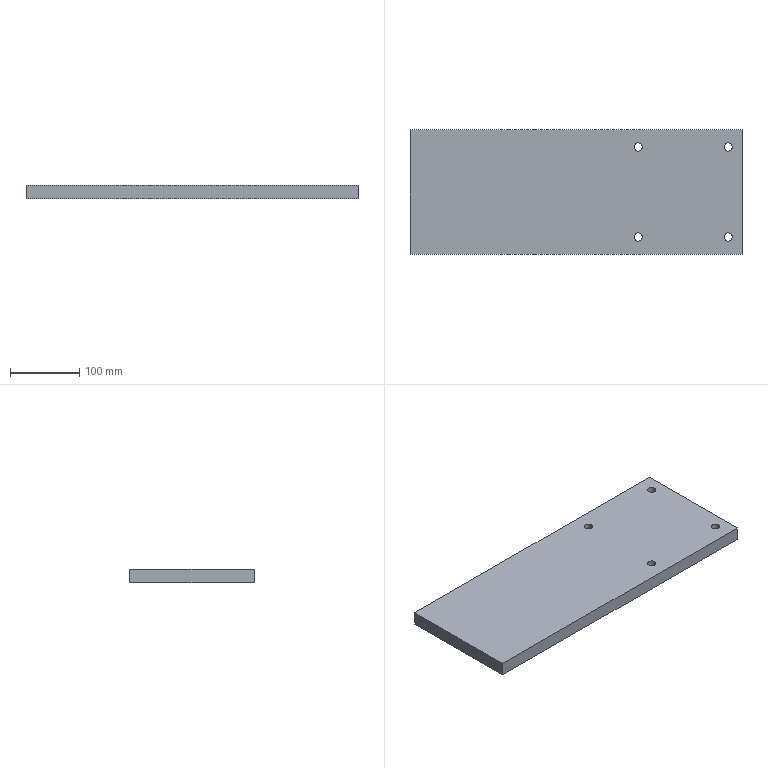Part | STEP file | Small Pad Plate 1 | 1 solid | 14 faces | box 480 x 180 x 20 mm | volume 1718952 mm3 | cylinder 8 | plane 6 | commonest cylinder face diameters 12 x8
STEP:
#1=CARTESIAN_POINT('',(0.,0.,0.));
#2=DIRECTION('',(0.,0.,1.));
#3=DIRECTION('',(1.,0.,0.));
#4=AXIS2_PLACEMENT_3D('',#1,#2,#3);
#5=CARTESIAN_POINT('',(96.,-65.,0.));
#6=VERTEX_POINT('',#5);
#7=CARTESIAN_POINT('',(96.,-65.,20.));
#8=VERTEX_POINT('',#7);
#9=CARTESIAN_POINT('',(96.,-65.,20.));
#10=DIRECTION('',(0.,0.,1.));
#11=VECTOR('',#10,1.);
#12=LINE('',#9,#11);
#13=CARTESIAN_POINT('',(90.,-65.,20.));
#14=DIRECTION('',(0.,0.,1.));
#15=DIRECTION('',(1.,0.,0.));
#16=AXIS2_PLACEMENT_3D('',#13,#14,#15);
#17=CYLINDRICAL_SURFACE('',#16,6.);
#18=CARTESIAN_POINT('',(6.283,0.));
#19=DIRECTION('',(0.,1.));
#20=VECTOR('',#19,1.);
#21=LINE('',#18,#20);
#22=(GEOMETRIC_REPRESENTATION_CONTEXT(2)PARAMETRIC_REPRESENTATION_CONTEXT()REPRESENTATION_CONTEXT('',''));
#23=DEFINITIONAL_REPRESENTATION('',(#21),#22);
#24=PCURVE('',#17,#23);
#25=CARTESIAN_POINT('',(90.,-65.,20.));
#26=DIRECTION('',(0.,0.,1.));
#27=DIRECTION('',(1.,0.,0.));
#28=AXIS2_PLACEMENT_3D('',#25,#26,#27);
#29=CYLINDRICAL_SURFACE('',#28,6.);
#30=CARTESIAN_POINT('',(0.,0.));
#31=DIRECTION('',(0.,1.));
#32=VECTOR('',#31,1.);
#33=LINE('',#30,#32);
#34=(GEOMETRIC_REPRESENTATION_CONTEXT(2)PARAMETRIC_REPRESENTATION_CONTEXT()REPRESENTATION_CONTEXT('',''));
#35=DEFINITIONAL_REPRESENTATION('',(#33),#34);
#36=PCURVE('',#29,#35);
#37=SURFACE_CURVE('',#12,(#24,#36),.PCURVE_S1.);
#38=EDGE_CURVE('',#6,#8,#37,.T.);
#39=ORIENTED_EDGE('',*,*,#38,.T.);
#40=CARTESIAN_POINT('',(84.,-65.,20.));
#41=VERTEX_POINT('',#40);
#42=CARTESIAN_POINT('',(90.,-65.,20.));
#43=DIRECTION('',(0.,0.,1.));
#44=DIRECTION('',(1.,0.,0.));
#45=AXIS2_PLACEMENT_3D('',#42,#43,#44);
#46=CIRCLE('',#45,6.);
#47=CARTESIAN_POINT('',(0.,0.));
#48=DIRECTION('',(1.,0.));
#49=VECTOR('',#48,1.);
#50=LINE('',#47,#49);
#51=(GEOMETRIC_REPRESENTATION_CONTEXT(2)PARAMETRIC_REPRESENTATION_CONTEXT()REPRESENTATION_CONTEXT('',''));
#52=DEFINITIONAL_REPRESENTATION('',(#50),#51);
#53=PCURVE('',#17,#52);
#54=CARTESIAN_POINT('',(0.,0.,20.));
#55=DIRECTION('',(0.,0.,1.));
#56=DIRECTION('',(1.,0.,0.));
#57=AXIS2_PLACEMENT_3D('',#54,#55,#56);
#58=PLANE('',#57);
#59=CARTESIAN_POINT('',(90.,-65.));
#60=DIRECTION('',(1.,0.));
#61=AXIS2_PLACEMENT_2D('',#59,#60);
#62=CIRCLE('',#61,6.);
#63=(GEOMETRIC_REPRESENTATION_CONTEXT(2)PARAMETRIC_REPRESENTATION_CONTEXT()REPRESENTATION_CONTEXT('',''));
#64=DEFINITIONAL_REPRESENTATION('',(#62),#63);
#65=PCURVE('',#58,#64);
#66=SURFACE_CURVE('',#46,(#53,#65),.PCURVE_S1.);
#67=EDGE_CURVE('',#41,#8,#66,.T.);
#68=ORIENTED_EDGE('',*,*,#67,.F.);
#69=CARTESIAN_POINT('',(84.,-65.,0.));
#70=VERTEX_POINT('',#69);
#71=CARTESIAN_POINT('',(84.,-65.,20.));
#72=DIRECTION('',(0.,0.,1.));
#73=VECTOR('',#72,1.);
#74=LINE('',#71,#73);
#75=CARTESIAN_POINT('',(3.142,0.));
#76=DIRECTION('',(0.,1.));
#77=VECTOR('',#76,1.);
#78=LINE('',#75,#77);
#79=(GEOMETRIC_REPRESENTATION_CONTEXT(2)PARAMETRIC_REPRESENTATION_CONTEXT()REPRESENTATION_CONTEXT('',''));
#80=DEFINITIONAL_REPRESENTATION('',(#78),#79);
#81=PCURVE('',#17,#80);
#82=CARTESIAN_POINT('',(3.142,0.));
#83=DIRECTION('',(0.,1.));
#84=VECTOR('',#83,1.);
#85=LINE('',#82,#84);
#86=(GEOMETRIC_REPRESENTATION_CONTEXT(2)PARAMETRIC_REPRESENTATION_CONTEXT()REPRESENTATION_CONTEXT('',''));
#87=DEFINITIONAL_REPRESENTATION('',(#85),#86);
#88=PCURVE('',#29,#87);
#89=SURFACE_CURVE('',#74,(#81,#88),.PCURVE_S1.);
#90=EDGE_CURVE('',#70,#41,#89,.T.);
#91=ORIENTED_EDGE('',*,*,#90,.F.);
#92=CARTESIAN_POINT('',(90.,-65.,0.));
#93=DIRECTION('',(0.,0.,1.));
#94=DIRECTION('',(1.,0.,0.));
#95=AXIS2_PLACEMENT_3D('',#92,#93,#94);
#96=CIRCLE('',#95,6.);
#97=CARTESIAN_POINT('',(0.,-20.));
#98=DIRECTION('',(1.,0.));
#99=VECTOR('',#98,1.);
#100=LINE('',#97,#99);
#101=(GEOMETRIC_REPRESENTATION_CONTEXT(2)PARAMETRIC_REPRESENTATION_CONTEXT()REPRESENTATION_CONTEXT('',''));
#102=DEFINITIONAL_REPRESENTATION('',(#100),#101);
#103=PCURVE('',#17,#102);
#104=CARTESIAN_POINT('',(0.,0.,0.));
#105=DIRECTION('',(0.,0.,1.));
#106=DIRECTION('',(1.,0.,0.));
#107=AXIS2_PLACEMENT_3D('',#104,#105,#106);
#108=PLANE('',#107);
#109=CARTESIAN_POINT('',(90.,-65.));
#110=DIRECTION('',(1.,0.));
#111=AXIS2_PLACEMENT_2D('',#109,#110);
#112=CIRCLE('',#111,6.);
#113=(GEOMETRIC_REPRESENTATION_CONTEXT(2)PARAMETRIC_REPRESENTATION_CONTEXT()REPRESENTATION_CONTEXT('',''));
#114=DEFINITIONAL_REPRESENTATION('',(#112),#113);
#115=PCURVE('',#108,#114);
#116=SURFACE_CURVE('',#96,(#103,#115),.PCURVE_S1.);
#117=EDGE_CURVE('',#70,#6,#116,.T.);
#118=ORIENTED_EDGE('',*,*,#117,.T.);
#119=EDGE_LOOP('',(#39,#68,#91,#118));
#120=FACE_BOUND('',#119,.F.);
#121=ADVANCED_FACE('',(#120),#17,.F.);
#122=CARTESIAN_POINT('',(96.,65.,0.));
#123=VERTEX_POINT('',#122);
#124=CARTESIAN_POINT('',(96.,65.,20.));
#125=VERTEX_POINT('',#124);
#126=CARTESIAN_POINT('',(96.,65.,20.));
#127=DIRECTION('',(0.,0.,1.));
#128=VECTOR('',#127,1.);
#129=LINE('',#126,#128);
#130=CARTESIAN_POINT('',(90.,65.,20.));
#131=DIRECTION('',(0.,0.,1.));
#132=DIRECTION('',(1.,0.,0.));
#133=AXIS2_PLACEMENT_3D('',#130,#131,#132);
#134=CYLINDRICAL_SURFACE('',#133,6.);
#135=CARTESIAN_POINT('',(6.283,0.));
#136=DIRECTION('',(0.,1.));
#137=VECTOR('',#136,1.);
#138=LINE('',#135,#137);
#139=(GEOMETRIC_REPRESENTATION_CONTEXT(2)PARAMETRIC_REPRESENTATION_CONTEXT()REPRESENTATION_CONTEXT('',''));
#140=DEFINITIONAL_REPRESENTATION('',(#138),#139);
#141=PCURVE('',#134,#140);
#142=CARTESIAN_POINT('',(90.,65.,20.));
#143=DIRECTION('',(0.,0.,1.));
#144=DIRECTION('',(1.,0.,0.));
#145=AXIS2_PLACEMENT_3D('',#142,#143,#144);
#146=CYLINDRICAL_SURFACE('',#145,6.);
#147=CARTESIAN_POINT('',(0.,0.));
#148=DIRECTION('',(0.,1.));
#149=VECTOR('',#148,1.);
#150=LINE('',#147,#149);
#151=(GEOMETRIC_REPRESENTATION_CONTEXT(2)PARAMETRIC_REPRESENTATION_CONTEXT()REPRESENTATION_CONTEXT('',''));
#152=DEFINITIONAL_REPRESENTATION('',(#150),#151);
#153=PCURVE('',#146,#152);
#154=SURFACE_CURVE('',#129,(#141,#153),.PCURVE_S1.);
#155=EDGE_CURVE('',#123,#125,#154,.T.);
#156=ORIENTED_EDGE('',*,*,#155,.T.);
#157=CARTESIAN_POINT('',(84.,65.,20.));
#158=VERTEX_POINT('',#157);
#159=CARTESIAN_POINT('',(90.,65.,20.));
#160=DIRECTION('',(0.,0.,1.));
#161=DIRECTION('',(1.,0.,0.));
#162=AXIS2_PLACEMENT_3D('',#159,#160,#161);
#163=CIRCLE('',#162,6.);
#164=CARTESIAN_POINT('',(0.,0.));
#165=DIRECTION('',(1.,0.));
#166=VECTOR('',#165,1.);
#167=LINE('',#164,#166);
#168=(GEOMETRIC_REPRESENTATION_CONTEXT(2)PARAMETRIC_REPRESENTATION_CONTEXT()REPRESENTATION_CONTEXT('',''));
#169=DEFINITIONAL_REPRESENTATION('',(#167),#168);
#170=PCURVE('',#134,#169);
#171=CARTESIAN_POINT('',(90.,65.));
#172=DIRECTION('',(1.,0.));
#173=AXIS2_PLACEMENT_2D('',#171,#172);
#174=CIRCLE('',#173,6.);
#175=(GEOMETRIC_REPRESENTATION_CONTEXT(2)PARAMETRIC_REPRESENTATION_CONTEXT()REPRESENTATION_CONTEXT('',''));
#176=DEFINITIONAL_REPRESENTATION('',(#174),#175);
#177=PCURVE('',#58,#176);
#178=SURFACE_CURVE('',#163,(#170,#177),.PCURVE_S1.);
#179=EDGE_CURVE('',#158,#125,#178,.T.);
#180=ORIENTED_EDGE('',*,*,#179,.F.);
#181=CARTESIAN_POINT('',(84.,65.,0.));
#182=VERTEX_POINT('',#181);
#183=CARTESIAN_POINT('',(84.,65.,20.));
#184=DIRECTION('',(0.,0.,1.));
#185=VECTOR('',#184,1.);
#186=LINE('',#183,#185);
#187=CARTESIAN_POINT('',(3.142,0.));
#188=DIRECTION('',(0.,1.));
#189=VECTOR('',#188,1.);
#190=LINE('',#187,#189);
#191=(GEOMETRIC_REPRESENTATION_CONTEXT(2)PARAMETRIC_REPRESENTATION_CONTEXT()REPRESENTATION_CONTEXT('',''));
#192=DEFINITIONAL_REPRESENTATION('',(#190),#191);
#193=PCURVE('',#134,#192);
#194=CARTESIAN_POINT('',(3.142,0.));
#195=DIRECTION('',(0.,1.));
#196=VECTOR('',#195,1.);
#197=LINE('',#194,#196);
#198=(GEOMETRIC_REPRESENTATION_CONTEXT(2)PARAMETRIC_REPRESENTATION_CONTEXT()REPRESENTATION_CONTEXT('',''));
#199=DEFINITIONAL_REPRESENTATION('',(#197),#198);
#200=PCURVE('',#146,#199);
#201=SURFACE_CURVE('',#186,(#193,#200),.PCURVE_S1.);
#202=EDGE_CURVE('',#182,#158,#201,.T.);
#203=ORIENTED_EDGE('',*,*,#202,.F.);
#204=CARTESIAN_POINT('',(90.,65.,0.));
#205=DIRECTION('',(0.,0.,1.));
#206=DIRECTION('',(1.,0.,0.));
#207=AXIS2_PLACEMENT_3D('',#204,#205,#206);
#208=CIRCLE('',#207,6.);
#209=CARTESIAN_POINT('',(0.,-20.));
#210=DIRECTION('',(1.,0.));
#211=VECTOR('',#210,1.);
#212=LINE('',#209,#211);
#213=(GEOMETRIC_REPRESENTATION_CONTEXT(2)PARAMETRIC_REPRESENTATION_CONTEXT()REPRESENTATION_CONTEXT('',''));
#214=DEFINITIONAL_REPRESENTATION('',(#212),#213);
#215=PCURVE('',#134,#214);
#216=CARTESIAN_POINT('',(90.,65.));
#217=DIRECTION('',(1.,0.));
#218=AXIS2_PLACEMENT_2D('',#216,#217);
#219=CIRCLE('',#218,6.);
#220=(GEOMETRIC_REPRESENTATION_CONTEXT(2)PARAMETRIC_REPRESENTATION_CONTEXT()REPRESENTATION_CONTEXT('',''));
#221=DEFINITIONAL_REPRESENTATION('',(#219),#220);
#222=PCURVE('',#108,#221);
#223=SURFACE_CURVE('',#208,(#215,#222),.PCURVE_S1.);
#224=EDGE_CURVE('',#182,#123,#223,.T.);
#225=ORIENTED_EDGE('',*,*,#224,.T.);
#226=EDGE_LOOP('',(#156,#180,#203,#225));
#227=FACE_BOUND('',#226,.F.);
#228=ADVANCED_FACE('',(#227),#134,.F.);
#229=CARTESIAN_POINT('',(226.,-65.,0.));
#230=VERTEX_POINT('',#229);
#231=CARTESIAN_POINT('',(226.,-65.,20.));
#232=VERTEX_POINT('',#231);
#233=CARTESIAN_POINT('',(226.,-65.,20.));
#234=DIRECTION('',(0.,0.,1.));
#235=VECTOR('',#234,1.);
#236=LINE('',#233,#235);
#237=CARTESIAN_POINT('',(220.,-65.,20.));
#238=DIRECTION('',(0.,0.,1.));
#239=DIRECTION('',(1.,0.,0.));
#240=AXIS2_PLACEMENT_3D('',#237,#238,#239);
#241=CYLINDRICAL_SURFACE('',#240,6.);
#242=CARTESIAN_POINT('',(6.283,0.));
#243=DIRECTION('',(0.,1.));
#244=VECTOR('',#243,1.);
#245=LINE('',#242,#244);
#246=(GEOMETRIC_REPRESENTATION_CONTEXT(2)PARAMETRIC_REPRESENTATION_CONTEXT()REPRESENTATION_CONTEXT('',''));
#247=DEFINITIONAL_REPRESENTATION('',(#245),#246);
#248=PCURVE('',#241,#247);
#249=CARTESIAN_POINT('',(220.,-65.,20.));
#250=DIRECTION('',(0.,0.,1.));
#251=DIRECTION('',(1.,0.,0.));
#252=AXIS2_PLACEMENT_3D('',#249,#250,#251);
#253=CYLINDRICAL_SURFACE('',#252,6.);
#254=CARTESIAN_POINT('',(0.,0.));
#255=DIRECTION('',(0.,1.));
#256=VECTOR('',#255,1.);
#257=LINE('',#254,#256);
#258=(GEOMETRIC_REPRESENTATION_CONTEXT(2)PARAMETRIC_REPRESENTATION_CONTEXT()REPRESENTATION_CONTEXT('',''));
#259=DEFINITIONAL_REPRESENTATION('',(#257),#258);
#260=PCURVE('',#253,#259);
#261=SURFACE_CURVE('',#236,(#248,#260),.PCURVE_S1.);
#262=EDGE_CURVE('',#230,#232,#261,.T.);
#263=ORIENTED_EDGE('',*,*,#262,.T.);
#264=CARTESIAN_POINT('',(214.,-65.,20.));
#265=VERTEX_POINT('',#264);
#266=CARTESIAN_POINT('',(220.,-65.,20.));
#267=DIRECTION('',(0.,0.,1.));
#268=DIRECTION('',(1.,0.,0.));
#269=AXIS2_PLACEMENT_3D('',#266,#267,#268);
#270=CIRCLE('',#269,6.);
#271=CARTESIAN_POINT('',(0.,0.));
#272=DIRECTION('',(1.,0.));
#273=VECTOR('',#272,1.);
#274=LINE('',#271,#273);
#275=(GEOMETRIC_REPRESENTATION_CONTEXT(2)PARAMETRIC_REPRESENTATION_CONTEXT()REPRESENTATION_CONTEXT('',''));
#276=DEFINITIONAL_REPRESENTATION('',(#274),#275);
#277=PCURVE('',#241,#276);
#278=CARTESIAN_POINT('',(220.,-65.));
#279=DIRECTION('',(1.,0.));
#280=AXIS2_PLACEMENT_2D('',#278,#279);
#281=CIRCLE('',#280,6.);
#282=(GEOMETRIC_REPRESENTATION_CONTEXT(2)PARAMETRIC_REPRESENTATION_CONTEXT()REPRESENTATION_CONTEXT('',''));
#283=DEFINITIONAL_REPRESENTATION('',(#281),#282);
#284=PCURVE('',#58,#283);
#285=SURFACE_CURVE('',#270,(#277,#284),.PCURVE_S1.);
#286=EDGE_CURVE('',#265,#232,#285,.T.);
#287=ORIENTED_EDGE('',*,*,#286,.F.);
#288=CARTESIAN_POINT('',(214.,-65.,0.));
#289=VERTEX_POINT('',#288);
#290=CARTESIAN_POINT('',(214.,-65.,20.));
#291=DIRECTION('',(0.,0.,1.));
#292=VECTOR('',#291,1.);
#293=LINE('',#290,#292);
#294=CARTESIAN_POINT('',(3.142,0.));
#295=DIRECTION('',(0.,1.));
#296=VECTOR('',#295,1.);
#297=LINE('',#294,#296);
#298=(GEOMETRIC_REPRESENTATION_CONTEXT(2)PARAMETRIC_REPRESENTATION_CONTEXT()REPRESENTATION_CONTEXT('',''));
#299=DEFINITIONAL_REPRESENTATION('',(#297),#298);
#300=PCURVE('',#241,#299);
#301=CARTESIAN_POINT('',(3.142,0.));
#302=DIRECTION('',(0.,1.));
#303=VECTOR('',#302,1.);
#304=LINE('',#301,#303);
#305=(GEOMETRIC_REPRESENTATION_CONTEXT(2)PARAMETRIC_REPRESENTATION_CONTEXT()REPRESENTATION_CONTEXT('',''));
#306=DEFINITIONAL_REPRESENTATION('',(#304),#305);
#307=PCURVE('',#253,#306);
#308=SURFACE_CURVE('',#293,(#300,#307),.PCURVE_S1.);
#309=EDGE_CURVE('',#289,#265,#308,.T.);
#310=ORIENTED_EDGE('',*,*,#309,.F.);
#311=CARTESIAN_POINT('',(220.,-65.,0.));
#312=DIRECTION('',(0.,0.,1.));
#313=DIRECTION('',(1.,0.,0.));
#314=AXIS2_PLACEMENT_3D('',#311,#312,#313);
#315=CIRCLE('',#314,6.);
#316=CARTESIAN_POINT('',(0.,-20.));
#317=DIRECTION('',(1.,0.));
#318=VECTOR('',#317,1.);
#319=LINE('',#316,#318);
#320=(GEOMETRIC_REPRESENTATION_CONTEXT(2)PARAMETRIC_REPRESENTATION_CONTEXT()REPRESENTATION_CONTEXT('',''));
#321=DEFINITIONAL_REPRESENTATION('',(#319),#320);
#322=PCURVE('',#241,#321);
#323=CARTESIAN_POINT('',(220.,-65.));
#324=DIRECTION('',(1.,0.));
#325=AXIS2_PLACEMENT_2D('',#323,#324);
#326=CIRCLE('',#325,6.);
#327=(GEOMETRIC_REPRESENTATION_CONTEXT(2)PARAMETRIC_REPRESENTATION_CONTEXT()REPRESENTATION_CONTEXT('',''));
#328=DEFINITIONAL_REPRESENTATION('',(#326),#327);
#329=PCURVE('',#108,#328);
#330=SURFACE_CURVE('',#315,(#322,#329),.PCURVE_S1.);
#331=EDGE_CURVE('',#289,#230,#330,.T.);
#332=ORIENTED_EDGE('',*,*,#331,.T.);
#333=EDGE_LOOP('',(#263,#287,#310,#332));
#334=FACE_BOUND('',#333,.F.);
#335=ADVANCED_FACE('',(#334),#241,.F.);
#336=CARTESIAN_POINT('',(226.,65.,0.));
#337=VERTEX_POINT('',#336);
#338=CARTESIAN_POINT('',(226.,65.,20.));
#339=VERTEX_POINT('',#338);
#340=CARTESIAN_POINT('',(226.,65.,20.));
#341=DIRECTION('',(0.,0.,1.));
#342=VECTOR('',#341,1.);
#343=LINE('',#340,#342);
#344=CARTESIAN_POINT('',(220.,65.,20.));
#345=DIRECTION('',(0.,0.,1.));
#346=DIRECTION('',(1.,0.,0.));
#347=AXIS2_PLACEMENT_3D('',#344,#345,#346);
#348=CYLINDRICAL_SURFACE('',#347,6.);
#349=CARTESIAN_POINT('',(6.283,0.));
#350=DIRECTION('',(0.,1.));
#351=VECTOR('',#350,1.);
#352=LINE('',#349,#351);
#353=(GEOMETRIC_REPRESENTATION_CONTEXT(2)PARAMETRIC_REPRESENTATION_CONTEXT()REPRESENTATION_CONTEXT('',''));
#354=DEFINITIONAL_REPRESENTATION('',(#352),#353);
#355=PCURVE('',#348,#354);
#356=CARTESIAN_POINT('',(220.,65.,20.));
#357=DIRECTION('',(0.,0.,1.));
#358=DIRECTION('',(1.,0.,0.));
#359=AXIS2_PLACEMENT_3D('',#356,#357,#358);
#360=CYLINDRICAL_SURFACE('',#359,6.);
#361=CARTESIAN_POINT('',(0.,0.));
#362=DIRECTION('',(0.,1.));
#363=VECTOR('',#362,1.);
#364=LINE('',#361,#363);
#365=(GEOMETRIC_REPRESENTATION_CONTEXT(2)PARAMETRIC_REPRESENTATION_CONTEXT()REPRESENTATION_CONTEXT('',''));
#366=DEFINITIONAL_REPRESENTATION('',(#364),#365);
#367=PCURVE('',#360,#366);
#368=SURFACE_CURVE('',#343,(#355,#367),.PCURVE_S1.);
#369=EDGE_CURVE('',#337,#339,#368,.T.);
#370=ORIENTED_EDGE('',*,*,#369,.T.);
#371=CARTESIAN_POINT('',(214.,65.,20.));
#372=VERTEX_POINT('',#371);
#373=CARTESIAN_POINT('',(220.,65.,20.));
#374=DIRECTION('',(0.,0.,1.));
#375=DIRECTION('',(1.,0.,0.));
#376=AXIS2_PLACEMENT_3D('',#373,#374,#375);
#377=CIRCLE('',#376,6.);
#378=CARTESIAN_POINT('',(0.,0.));
#379=DIRECTION('',(1.,0.));
#380=VECTOR('',#379,1.);
#381=LINE('',#378,#380);
#382=(GEOMETRIC_REPRESENTATION_CONTEXT(2)PARAMETRIC_REPRESENTATION_CONTEXT()REPRESENTATION_CONTEXT('',''));
#383=DEFINITIONAL_REPRESENTATION('',(#381),#382);
#384=PCURVE('',#348,#383);
#385=CARTESIAN_POINT('',(220.,65.));
#386=DIRECTION('',(1.,0.));
#387=AXIS2_PLACEMENT_2D('',#385,#386);
#388=CIRCLE('',#387,6.);
#389=(GEOMETRIC_REPRESENTATION_CONTEXT(2)PARAMETRIC_REPRESENTATION_CONTEXT()REPRESENTATION_CONTEXT('',''));
#390=DEFINITIONAL_REPRESENTATION('',(#388),#389);
#391=PCURVE('',#58,#390);
#392=SURFACE_CURVE('',#377,(#384,#391),.PCURVE_S1.);
#393=EDGE_CURVE('',#372,#339,#392,.T.);
#394=ORIENTED_EDGE('',*,*,#393,.F.);
#395=CARTESIAN_POINT('',(214.,65.,0.));
#396=VERTEX_POINT('',#395);
#397=CARTESIAN_POINT('',(214.,65.,20.));
#398=DIRECTION('',(0.,0.,1.));
#399=VECTOR('',#398,1.);
#400=LINE('',#397,#399);
#401=CARTESIAN_POINT('',(3.142,0.));
#402=DIRECTION('',(0.,1.));
#403=VECTOR('',#402,1.);
#404=LINE('',#401,#403);
#405=(GEOMETRIC_REPRESENTATION_CONTEXT(2)PARAMETRIC_REPRESENTATION_CONTEXT()REPRESENTATION_CONTEXT('',''));
#406=DEFINITIONAL_REPRESENTATION('',(#404),#405);
#407=PCURVE('',#348,#406);
#408=CARTESIAN_POINT('',(3.142,0.));
#409=DIRECTION('',(0.,1.));
#410=VECTOR('',#409,1.);
#411=LINE('',#408,#410);
#412=(GEOMETRIC_REPRESENTATION_CONTEXT(2)PARAMETRIC_REPRESENTATION_CONTEXT()REPRESENTATION_CONTEXT('',''));
#413=DEFINITIONAL_REPRESENTATION('',(#411),#412);
#414=PCURVE('',#360,#413);
#415=SURFACE_CURVE('',#400,(#407,#414),.PCURVE_S1.);
#416=EDGE_CURVE('',#396,#372,#415,.T.);
#417=ORIENTED_EDGE('',*,*,#416,.F.);
#418=CARTESIAN_POINT('',(220.,65.,0.));
#419=DIRECTION('',(0.,0.,1.));
#420=DIRECTION('',(1.,0.,0.));
#421=AXIS2_PLACEMENT_3D('',#418,#419,#420);
#422=CIRCLE('',#421,6.);
#423=CARTESIAN_POINT('',(0.,-20.));
#424=DIRECTION('',(1.,0.));
#425=VECTOR('',#424,1.);
#426=LINE('',#423,#425);
#427=(GEOMETRIC_REPRESENTATION_CONTEXT(2)PARAMETRIC_REPRESENTATION_CONTEXT()REPRESENTATION_CONTEXT('',''));
#428=DEFINITIONAL_REPRESENTATION('',(#426),#427);
#429=PCURVE('',#348,#428);
#430=CARTESIAN_POINT('',(220.,65.));
#431=DIRECTION('',(1.,0.));
#432=AXIS2_PLACEMENT_2D('',#430,#431);
#433=CIRCLE('',#432,6.);
#434=(GEOMETRIC_REPRESENTATION_CONTEXT(2)PARAMETRIC_REPRESENTATION_CONTEXT()REPRESENTATION_CONTEXT('',''));
#435=DEFINITIONAL_REPRESENTATION('',(#433),#434);
#436=PCURVE('',#108,#435);
#437=SURFACE_CURVE('',#422,(#429,#436),.PCURVE_S1.);
#438=EDGE_CURVE('',#396,#337,#437,.T.);
#439=ORIENTED_EDGE('',*,*,#438,.T.);
#440=EDGE_LOOP('',(#370,#394,#417,#439));
#441=FACE_BOUND('',#440,.F.);
#442=ADVANCED_FACE('',(#441),#348,.F.);
#443=CARTESIAN_POINT('',(240.,-90.,0.));
#444=VERTEX_POINT('',#443);
#445=CARTESIAN_POINT('',(240.,90.,0.));
#446=VERTEX_POINT('',#445);
#447=CARTESIAN_POINT('',(240.,90.,0.));
#448=DIRECTION('',(0.,1.,0.));
#449=VECTOR('',#448,1.);
#450=LINE('',#447,#449);
#451=CARTESIAN_POINT('',(240.,90.,20.));
#452=DIRECTION('',(-1.,0.,0.));
#453=DIRECTION('',(0.,-1.,0.));
#454=AXIS2_PLACEMENT_3D('',#451,#452,#453);
#455=PLANE('',#454);
#456=CARTESIAN_POINT('',(0.,-20.));
#457=DIRECTION('',(-1.,0.));
#458=VECTOR('',#457,1.);
#459=LINE('',#456,#458);
#460=(GEOMETRIC_REPRESENTATION_CONTEXT(2)PARAMETRIC_REPRESENTATION_CONTEXT()REPRESENTATION_CONTEXT('',''));
#461=DEFINITIONAL_REPRESENTATION('',(#459),#460);
#462=PCURVE('',#455,#461);
#463=CARTESIAN_POINT('',(240.,90.));
#464=DIRECTION('',(0.,1.));
#465=VECTOR('',#464,1.);
#466=LINE('',#463,#465);
#467=(GEOMETRIC_REPRESENTATION_CONTEXT(2)PARAMETRIC_REPRESENTATION_CONTEXT()REPRESENTATION_CONTEXT('',''));
#468=DEFINITIONAL_REPRESENTATION('',(#466),#467);
#469=PCURVE('',#108,#468);
#470=SURFACE_CURVE('',#450,(#462,#469),.PCURVE_S1.);
#471=EDGE_CURVE('',#444,#446,#470,.T.);
#472=ORIENTED_EDGE('',*,*,#471,.T.);
#473=CARTESIAN_POINT('',(240.,90.,20.));
#474=VERTEX_POINT('',#473);
#475=CARTESIAN_POINT('',(240.,90.,20.));
#476=DIRECTION('',(0.,0.,-1.));
#477=VECTOR('',#476,1.);
#478=LINE('',#475,#477);
#479=CARTESIAN_POINT('',(0.,0.));
#480=DIRECTION('',(0.,-1.));
#481=VECTOR('',#480,1.);
#482=LINE('',#479,#481);
#483=(GEOMETRIC_REPRESENTATION_CONTEXT(2)PARAMETRIC_REPRESENTATION_CONTEXT()REPRESENTATION_CONTEXT('',''));
#484=DEFINITIONAL_REPRESENTATION('',(#482),#483);
#485=PCURVE('',#455,#484);
#486=CARTESIAN_POINT('',(-240.,90.,20.));
#487=DIRECTION('',(0.,-1.,0.));
#488=DIRECTION('',(0.,0.,-1.));
#489=AXIS2_PLACEMENT_3D('',#486,#487,#488);
#490=PLANE('',#489);
#491=CARTESIAN_POINT('',(0.,480.));
#492=DIRECTION('',(1.,0.));
#493=VECTOR('',#492,1.);
#494=LINE('',#491,#493);
#495=(GEOMETRIC_REPRESENTATION_CONTEXT(2)PARAMETRIC_REPRESENTATION_CONTEXT()REPRESENTATION_CONTEXT('',''));
#496=DEFINITIONAL_REPRESENTATION('',(#494),#495);
#497=PCURVE('',#490,#496);
#498=SURFACE_CURVE('',#478,(#485,#497),.PCURVE_S1.);
#499=EDGE_CURVE('',#474,#446,#498,.T.);
#500=ORIENTED_EDGE('',*,*,#499,.F.);
#501=CARTESIAN_POINT('',(240.,-90.,20.));
#502=VERTEX_POINT('',#501);
#503=CARTESIAN_POINT('',(240.,90.,20.));
#504=DIRECTION('',(0.,1.,0.));
#505=VECTOR('',#504,1.);
#506=LINE('',#503,#505);
#507=CARTESIAN_POINT('',(0.,0.));
#508=DIRECTION('',(-1.,0.));
#509=VECTOR('',#508,1.);
#510=LINE('',#507,#509);
#511=(GEOMETRIC_REPRESENTATION_CONTEXT(2)PARAMETRIC_REPRESENTATION_CONTEXT()REPRESENTATION_CONTEXT('',''));
#512=DEFINITIONAL_REPRESENTATION('',(#510),#511);
#513=PCURVE('',#455,#512);
#514=CARTESIAN_POINT('',(240.,90.));
#515=DIRECTION('',(0.,1.));
#516=VECTOR('',#515,1.);
#517=LINE('',#514,#516);
#518=(GEOMETRIC_REPRESENTATION_CONTEXT(2)PARAMETRIC_REPRESENTATION_CONTEXT()REPRESENTATION_CONTEXT('',''));
#519=DEFINITIONAL_REPRESENTATION('',(#517),#518);
#520=PCURVE('',#58,#519);
#521=SURFACE_CURVE('',#506,(#513,#520),.PCURVE_S1.);
#522=EDGE_CURVE('',#502,#474,#521,.T.);
#523=ORIENTED_EDGE('',*,*,#522,.F.);
#524=CARTESIAN_POINT('',(240.,-90.,20.));
#525=DIRECTION('',(0.,0.,-1.));
#526=VECTOR('',#525,1.);
#527=LINE('',#524,#526);
#528=CARTESIAN_POINT('',(180.,0.));
#529=DIRECTION('',(0.,-1.));
#530=VECTOR('',#529,1.);
#531=LINE('',#528,#530);
#532=(GEOMETRIC_REPRESENTATION_CONTEXT(2)PARAMETRIC_REPRESENTATION_CONTEXT()REPRESENTATION_CONTEXT('',''));
#533=DEFINITIONAL_REPRESENTATION('',(#531),#532);
#534=PCURVE('',#455,#533);
#535=CARTESIAN_POINT('',(-240.,-90.,20.));
#536=DIRECTION('',(0.,1.,0.));
#537=DIRECTION('',(0.,0.,1.));
#538=AXIS2_PLACEMENT_3D('',#535,#536,#537);
#539=PLANE('',#538);
#540=CARTESIAN_POINT('',(0.,480.));
#541=DIRECTION('',(-1.,0.));
#542=VECTOR('',#541,1.);
#543=LINE('',#540,#542);
#544=(GEOMETRIC_REPRESENTATION_CONTEXT(2)PARAMETRIC_REPRESENTATION_CONTEXT()REPRESENTATION_CONTEXT('',''));
#545=DEFINITIONAL_REPRESENTATION('',(#543),#544);
#546=PCURVE('',#539,#545);
#547=SURFACE_CURVE('',#527,(#534,#546),.PCURVE_S1.);
#548=EDGE_CURVE('',#502,#444,#547,.T.);
#549=ORIENTED_EDGE('',*,*,#548,.T.);
#550=EDGE_LOOP('',(#472,#500,#523,#549));
#551=FACE_BOUND('',#550,.T.);
#552=ADVANCED_FACE('',(#551),#455,.F.);
#553=CARTESIAN_POINT('',(-240.,90.,0.));
#554=VERTEX_POINT('',#553);
#555=CARTESIAN_POINT('',(-240.,90.,0.));
#556=DIRECTION('',(-1.,0.,0.));
#557=VECTOR('',#556,1.);
#558=LINE('',#555,#557);
#559=CARTESIAN_POINT('',(20.,0.));
#560=DIRECTION('',(0.,-1.));
#561=VECTOR('',#560,1.);
#562=LINE('',#559,#561);
#563=(GEOMETRIC_REPRESENTATION_CONTEXT(2)PARAMETRIC_REPRESENTATION_CONTEXT()REPRESENTATION_CONTEXT('',''));
#564=DEFINITIONAL_REPRESENTATION('',(#562),#563);
#565=PCURVE('',#490,#564);
#566=CARTESIAN_POINT('',(-240.,90.));
#567=DIRECTION('',(-1.,0.));
#568=VECTOR('',#567,1.);
#569=LINE('',#566,#568);
#570=(GEOMETRIC_REPRESENTATION_CONTEXT(2)PARAMETRIC_REPRESENTATION_CONTEXT()REPRESENTATION_CONTEXT('',''));
#571=DEFINITIONAL_REPRESENTATION('',(#569),#570);
#572=PCURVE('',#108,#571);
#573=SURFACE_CURVE('',#558,(#565,#572),.PCURVE_S1.);
#574=EDGE_CURVE('',#446,#554,#573,.T.);
#575=ORIENTED_EDGE('',*,*,#574,.T.);
#576=CARTESIAN_POINT('',(-240.,90.,20.));
#577=VERTEX_POINT('',#576);
#578=CARTESIAN_POINT('',(-240.,90.,20.));
#579=DIRECTION('',(0.,0.,-1.));
#580=VECTOR('',#579,1.);
#581=LINE('',#578,#580);
#582=CARTESIAN_POINT('',(0.,0.));
#583=DIRECTION('',(1.,0.));
#584=VECTOR('',#583,1.);
#585=LINE('',#582,#584);
#586=(GEOMETRIC_REPRESENTATION_CONTEXT(2)PARAMETRIC_REPRESENTATION_CONTEXT()REPRESENTATION_CONTEXT('',''));
#587=DEFINITIONAL_REPRESENTATION('',(#585),#586);
#588=PCURVE('',#490,#587);
#589=CARTESIAN_POINT('',(-240.,90.,20.));
#590=DIRECTION('',(1.,0.,0.));
#591=DIRECTION('',(0.,1.,0.));
#592=AXIS2_PLACEMENT_3D('',#589,#590,#591);
#593=PLANE('',#592);
#594=CARTESIAN_POINT('',(0.,0.));
#595=DIRECTION('',(0.,-1.));
#596=VECTOR('',#595,1.);
#597=LINE('',#594,#596);
#598=(GEOMETRIC_REPRESENTATION_CONTEXT(2)PARAMETRIC_REPRESENTATION_CONTEXT()REPRESENTATION_CONTEXT('',''));
#599=DEFINITIONAL_REPRESENTATION('',(#597),#598);
#600=PCURVE('',#593,#599);
#601=SURFACE_CURVE('',#581,(#588,#600),.PCURVE_S1.);
#602=EDGE_CURVE('',#577,#554,#601,.T.);
#603=ORIENTED_EDGE('',*,*,#602,.F.);
#604=CARTESIAN_POINT('',(-240.,90.,20.));
#605=DIRECTION('',(-1.,0.,0.));
#606=VECTOR('',#605,1.);
#607=LINE('',#604,#606);
#608=CARTESIAN_POINT('',(0.,0.));
#609=DIRECTION('',(0.,-1.));
#610=VECTOR('',#609,1.);
#611=LINE('',#608,#610);
#612=(GEOMETRIC_REPRESENTATION_CONTEXT(2)PARAMETRIC_REPRESENTATION_CONTEXT()REPRESENTATION_CONTEXT('',''));
#613=DEFINITIONAL_REPRESENTATION('',(#611),#612);
#614=PCURVE('',#490,#613);
#615=CARTESIAN_POINT('',(-240.,90.));
#616=DIRECTION('',(-1.,0.));
#617=VECTOR('',#616,1.);
#618=LINE('',#615,#617);
#619=(GEOMETRIC_REPRESENTATION_CONTEXT(2)PARAMETRIC_REPRESENTATION_CONTEXT()REPRESENTATION_CONTEXT('',''));
#620=DEFINITIONAL_REPRESENTATION('',(#618),#619);
#621=PCURVE('',#58,#620);
#622=SURFACE_CURVE('',#607,(#614,#621),.PCURVE_S1.);
#623=EDGE_CURVE('',#474,#577,#622,.T.);
#624=ORIENTED_EDGE('',*,*,#623,.F.);
#625=ORIENTED_EDGE('',*,*,#499,.T.);
#626=EDGE_LOOP('',(#575,#603,#624,#625));
#627=FACE_BOUND('',#626,.T.);
#628=ADVANCED_FACE('',(#627),#490,.F.);
#629=CARTESIAN_POINT('',(-240.,-90.,0.));
#630=VERTEX_POINT('',#629);
#631=CARTESIAN_POINT('',(-240.,90.,0.));
#632=DIRECTION('',(0.,-1.,0.));
#633=VECTOR('',#632,1.);
#634=LINE('',#631,#633);
#635=CARTESIAN_POINT('',(0.,-20.));
#636=DIRECTION('',(-1.,0.));
#637=VECTOR('',#636,1.);
#638=LINE('',#635,#637);
#639=(GEOMETRIC_REPRESENTATION_CONTEXT(2)PARAMETRIC_REPRESENTATION_CONTEXT()REPRESENTATION_CONTEXT('',''));
#640=DEFINITIONAL_REPRESENTATION('',(#638),#639);
#641=PCURVE('',#593,#640);
#642=CARTESIAN_POINT('',(-240.,90.));
#643=DIRECTION('',(0.,-1.));
#644=VECTOR('',#643,1.);
#645=LINE('',#642,#644);
#646=(GEOMETRIC_REPRESENTATION_CONTEXT(2)PARAMETRIC_REPRESENTATION_CONTEXT()REPRESENTATION_CONTEXT('',''));
#647=DEFINITIONAL_REPRESENTATION('',(#645),#646);
#648=PCURVE('',#108,#647);
#649=SURFACE_CURVE('',#634,(#641,#648),.PCURVE_S1.);
#650=EDGE_CURVE('',#554,#630,#649,.T.);
#651=ORIENTED_EDGE('',*,*,#650,.T.);
#652=CARTESIAN_POINT('',(-240.,-90.,20.));
#653=VERTEX_POINT('',#652);
#654=CARTESIAN_POINT('',(-240.,-90.,20.));
#655=DIRECTION('',(0.,0.,-1.));
#656=VECTOR('',#655,1.);
#657=LINE('',#654,#656);
#658=CARTESIAN_POINT('',(-180.,0.));
#659=DIRECTION('',(0.,-1.));
#660=VECTOR('',#659,1.);
#661=LINE('',#658,#660);
#662=(GEOMETRIC_REPRESENTATION_CONTEXT(2)PARAMETRIC_REPRESENTATION_CONTEXT()REPRESENTATION_CONTEXT('',''));
#663=DEFINITIONAL_REPRESENTATION('',(#661),#662);
#664=PCURVE('',#593,#663);
#665=CARTESIAN_POINT('',(0.,0.));
#666=DIRECTION('',(-1.,0.));
#667=VECTOR('',#666,1.);
#668=LINE('',#665,#667);
#669=(GEOMETRIC_REPRESENTATION_CONTEXT(2)PARAMETRIC_REPRESENTATION_CONTEXT()REPRESENTATION_CONTEXT('',''));
#670=DEFINITIONAL_REPRESENTATION('',(#668),#669);
#671=PCURVE('',#539,#670);
#672=SURFACE_CURVE('',#657,(#664,#671),.PCURVE_S1.);
#673=EDGE_CURVE('',#653,#630,#672,.T.);
#674=ORIENTED_EDGE('',*,*,#673,.F.);
#675=CARTESIAN_POINT('',(-240.,90.,20.));
#676=DIRECTION('',(0.,-1.,0.));
#677=VECTOR('',#676,1.);
#678=LINE('',#675,#677);
#679=CARTESIAN_POINT('',(0.,0.));
#680=DIRECTION('',(-1.,0.));
#681=VECTOR('',#680,1.);
#682=LINE('',#679,#681);
#683=(GEOMETRIC_REPRESENTATION_CONTEXT(2)PARAMETRIC_REPRESENTATION_CONTEXT()REPRESENTATION_CONTEXT('',''));
#684=DEFINITIONAL_REPRESENTATION('',(#682),#683);
#685=PCURVE('',#593,#684);
#686=CARTESIAN_POINT('',(-240.,90.));
#687=DIRECTION('',(0.,-1.));
#688=VECTOR('',#687,1.);
#689=LINE('',#686,#688);
#690=(GEOMETRIC_REPRESENTATION_CONTEXT(2)PARAMETRIC_REPRESENTATION_CONTEXT()REPRESENTATION_CONTEXT('',''));
#691=DEFINITIONAL_REPRESENTATION('',(#689),#690);
#692=PCURVE('',#58,#691);
#693=SURFACE_CURVE('',#678,(#685,#692),.PCURVE_S1.);
#694=EDGE_CURVE('',#577,#653,#693,.T.);
#695=ORIENTED_EDGE('',*,*,#694,.F.);
#696=ORIENTED_EDGE('',*,*,#602,.T.);
#697=EDGE_LOOP('',(#651,#674,#695,#696));
#698=FACE_BOUND('',#697,.T.);
#699=ADVANCED_FACE('',(#698),#593,.F.);
#700=CARTESIAN_POINT('',(-240.,-90.,0.));
#701=DIRECTION('',(1.,0.,0.));
#702=VECTOR('',#701,1.);
#703=LINE('',#700,#702);
#704=CARTESIAN_POINT('',(-20.,0.));
#705=DIRECTION('',(0.,1.));
#706=VECTOR('',#705,1.);
#707=LINE('',#704,#706);
#708=(GEOMETRIC_REPRESENTATION_CONTEXT(2)PARAMETRIC_REPRESENTATION_CONTEXT()REPRESENTATION_CONTEXT('',''));
#709=DEFINITIONAL_REPRESENTATION('',(#707),#708);
#710=PCURVE('',#539,#709);
#711=CARTESIAN_POINT('',(-240.,-90.));
#712=DIRECTION('',(1.,0.));
#713=VECTOR('',#712,1.);
#714=LINE('',#711,#713);
#715=(GEOMETRIC_REPRESENTATION_CONTEXT(2)PARAMETRIC_REPRESENTATION_CONTEXT()REPRESENTATION_CONTEXT('',''));
#716=DEFINITIONAL_REPRESENTATION('',(#714),#715);
#717=PCURVE('',#108,#716);
#718=SURFACE_CURVE('',#703,(#710,#717),.PCURVE_S1.);
#719=EDGE_CURVE('',#630,#444,#718,.T.);
#720=ORIENTED_EDGE('',*,*,#719,.T.);
#721=ORIENTED_EDGE('',*,*,#548,.F.);
#722=CARTESIAN_POINT('',(-240.,-90.,20.));
#723=DIRECTION('',(1.,0.,0.));
#724=VECTOR('',#723,1.);
#725=LINE('',#722,#724);
#726=CARTESIAN_POINT('',(0.,0.));
#727=DIRECTION('',(0.,1.));
#728=VECTOR('',#727,1.);
#729=LINE('',#726,#728);
#730=(GEOMETRIC_REPRESENTATION_CONTEXT(2)PARAMETRIC_REPRESENTATION_CONTEXT()REPRESENTATION_CONTEXT('',''));
#731=DEFINITIONAL_REPRESENTATION('',(#729),#730);
#732=PCURVE('',#539,#731);
#733=CARTESIAN_POINT('',(-240.,-90.));
#734=DIRECTION('',(1.,0.));
#735=VECTOR('',#734,1.);
#736=LINE('',#733,#735);
#737=(GEOMETRIC_REPRESENTATION_CONTEXT(2)PARAMETRIC_REPRESENTATION_CONTEXT()REPRESENTATION_CONTEXT('',''));
#738=DEFINITIONAL_REPRESENTATION('',(#736),#737);
#739=PCURVE('',#58,#738);
#740=SURFACE_CURVE('',#725,(#732,#739),.PCURVE_S1.);
#741=EDGE_CURVE('',#653,#502,#740,.T.);
#742=ORIENTED_EDGE('',*,*,#741,.F.);
#743=ORIENTED_EDGE('',*,*,#673,.T.);
#744=EDGE_LOOP('',(#720,#721,#742,#743));
#745=FACE_BOUND('',#744,.T.);
#746=ADVANCED_FACE('',(#745),#539,.F.);
#747=CARTESIAN_POINT('',(90.,-65.,20.));
#748=DIRECTION('',(0.,0.,1.));
#749=DIRECTION('',(1.,0.,0.));
#750=AXIS2_PLACEMENT_3D('',#747,#748,#749);
#751=CIRCLE('',#750,6.);
#752=CARTESIAN_POINT('',(90.,-65.));
#753=DIRECTION('',(1.,0.));
#754=AXIS2_PLACEMENT_2D('',#752,#753);
#755=CIRCLE('',#754,6.);
#756=(GEOMETRIC_REPRESENTATION_CONTEXT(2)PARAMETRIC_REPRESENTATION_CONTEXT()REPRESENTATION_CONTEXT('',''));
#757=DEFINITIONAL_REPRESENTATION('',(#755),#756);
#758=PCURVE('',#58,#757);
#759=CARTESIAN_POINT('',(0.,0.));
#760=DIRECTION('',(1.,0.));
#761=VECTOR('',#760,1.);
#762=LINE('',#759,#761);
#763=(GEOMETRIC_REPRESENTATION_CONTEXT(2)PARAMETRIC_REPRESENTATION_CONTEXT()REPRESENTATION_CONTEXT('',''));
#764=DEFINITIONAL_REPRESENTATION('',(#762),#763);
#765=PCURVE('',#29,#764);
#766=SURFACE_CURVE('',#751,(#758,#765),.PCURVE_S1.);
#767=EDGE_CURVE('',#8,#41,#766,.T.);
#768=ORIENTED_EDGE('',*,*,#767,.F.);
#769=ORIENTED_EDGE('',*,*,#67,.F.);
#770=EDGE_LOOP('',(#768,#769));
#771=FACE_BOUND('',#770,.T.);
#772=CARTESIAN_POINT('',(90.,65.,20.));
#773=DIRECTION('',(0.,0.,1.));
#774=DIRECTION('',(1.,0.,0.));
#775=AXIS2_PLACEMENT_3D('',#772,#773,#774);
#776=CIRCLE('',#775,6.);
#777=CARTESIAN_POINT('',(90.,65.));
#778=DIRECTION('',(1.,0.));
#779=AXIS2_PLACEMENT_2D('',#777,#778);
#780=CIRCLE('',#779,6.);
#781=(GEOMETRIC_REPRESENTATION_CONTEXT(2)PARAMETRIC_REPRESENTATION_CONTEXT()REPRESENTATION_CONTEXT('',''));
#782=DEFINITIONAL_REPRESENTATION('',(#780),#781);
#783=PCURVE('',#58,#782);
#784=CARTESIAN_POINT('',(0.,0.));
#785=DIRECTION('',(1.,0.));
#786=VECTOR('',#785,1.);
#787=LINE('',#784,#786);
#788=(GEOMETRIC_REPRESENTATION_CONTEXT(2)PARAMETRIC_REPRESENTATION_CONTEXT()REPRESENTATION_CONTEXT('',''));
#789=DEFINITIONAL_REPRESENTATION('',(#787),#788);
#790=PCURVE('',#146,#789);
#791=SURFACE_CURVE('',#776,(#783,#790),.PCURVE_S1.);
#792=EDGE_CURVE('',#125,#158,#791,.T.);
#793=ORIENTED_EDGE('',*,*,#792,.F.);
#794=ORIENTED_EDGE('',*,*,#179,.F.);
#795=EDGE_LOOP('',(#793,#794));
#796=FACE_BOUND('',#795,.T.);
#797=CARTESIAN_POINT('',(220.,-65.,20.));
#798=DIRECTION('',(0.,0.,1.));
#799=DIRECTION('',(1.,0.,0.));
#800=AXIS2_PLACEMENT_3D('',#797,#798,#799);
#801=CIRCLE('',#800,6.);
#802=CARTESIAN_POINT('',(220.,-65.));
#803=DIRECTION('',(1.,0.));
#804=AXIS2_PLACEMENT_2D('',#802,#803);
#805=CIRCLE('',#804,6.);
#806=(GEOMETRIC_REPRESENTATION_CONTEXT(2)PARAMETRIC_REPRESENTATION_CONTEXT()REPRESENTATION_CONTEXT('',''));
#807=DEFINITIONAL_REPRESENTATION('',(#805),#806);
#808=PCURVE('',#58,#807);
#809=CARTESIAN_POINT('',(0.,0.));
#810=DIRECTION('',(1.,0.));
#811=VECTOR('',#810,1.);
#812=LINE('',#809,#811);
#813=(GEOMETRIC_REPRESENTATION_CONTEXT(2)PARAMETRIC_REPRESENTATION_CONTEXT()REPRESENTATION_CONTEXT('',''));
#814=DEFINITIONAL_REPRESENTATION('',(#812),#813);
#815=PCURVE('',#253,#814);
#816=SURFACE_CURVE('',#801,(#808,#815),.PCURVE_S1.);
#817=EDGE_CURVE('',#232,#265,#816,.T.);
#818=ORIENTED_EDGE('',*,*,#817,.F.);
#819=ORIENTED_EDGE('',*,*,#286,.F.);
#820=EDGE_LOOP('',(#818,#819));
#821=FACE_BOUND('',#820,.T.);
#822=CARTESIAN_POINT('',(220.,65.,20.));
#823=DIRECTION('',(0.,0.,1.));
#824=DIRECTION('',(1.,0.,0.));
#825=AXIS2_PLACEMENT_3D('',#822,#823,#824);
#826=CIRCLE('',#825,6.);
#827=CARTESIAN_POINT('',(220.,65.));
#828=DIRECTION('',(1.,0.));
#829=AXIS2_PLACEMENT_2D('',#827,#828);
#830=CIRCLE('',#829,6.);
#831=(GEOMETRIC_REPRESENTATION_CONTEXT(2)PARAMETRIC_REPRESENTATION_CONTEXT()REPRESENTATION_CONTEXT('',''));
#832=DEFINITIONAL_REPRESENTATION('',(#830),#831);
#833=PCURVE('',#58,#832);
#834=CARTESIAN_POINT('',(0.,0.));
#835=DIRECTION('',(1.,0.));
#836=VECTOR('',#835,1.);
#837=LINE('',#834,#836);
#838=(GEOMETRIC_REPRESENTATION_CONTEXT(2)PARAMETRIC_REPRESENTATION_CONTEXT()REPRESENTATION_CONTEXT('',''));
#839=DEFINITIONAL_REPRESENTATION('',(#837),#838);
#840=PCURVE('',#360,#839);
#841=SURFACE_CURVE('',#826,(#833,#840),.PCURVE_S1.);
#842=EDGE_CURVE('',#339,#372,#841,.T.);
#843=ORIENTED_EDGE('',*,*,#842,.F.);
#844=ORIENTED_EDGE('',*,*,#393,.F.);
#845=EDGE_LOOP('',(#843,#844));
#846=FACE_BOUND('',#845,.T.);
#847=ORIENTED_EDGE('',*,*,#522,.T.);
#848=ORIENTED_EDGE('',*,*,#623,.T.);
#849=ORIENTED_EDGE('',*,*,#694,.T.);
#850=ORIENTED_EDGE('',*,*,#741,.T.);
#851=EDGE_LOOP('',(#847,#848,#849,#850));
#852=FACE_BOUND('',#851,.T.);
#853=ADVANCED_FACE('',(#771,#796,#821,#846,#852),#58,.T.);
#854=CARTESIAN_POINT('',(90.,-65.,0.));
#855=DIRECTION('',(0.,0.,1.));
#856=DIRECTION('',(1.,0.,0.));
#857=AXIS2_PLACEMENT_3D('',#854,#855,#856);
#858=CIRCLE('',#857,6.);
#859=CARTESIAN_POINT('',(90.,-65.));
#860=DIRECTION('',(1.,0.));
#861=AXIS2_PLACEMENT_2D('',#859,#860);
#862=CIRCLE('',#861,6.);
#863=(GEOMETRIC_REPRESENTATION_CONTEXT(2)PARAMETRIC_REPRESENTATION_CONTEXT()REPRESENTATION_CONTEXT('',''));
#864=DEFINITIONAL_REPRESENTATION('',(#862),#863);
#865=PCURVE('',#108,#864);
#866=CARTESIAN_POINT('',(0.,-20.));
#867=DIRECTION('',(1.,0.));
#868=VECTOR('',#867,1.);
#869=LINE('',#866,#868);
#870=(GEOMETRIC_REPRESENTATION_CONTEXT(2)PARAMETRIC_REPRESENTATION_CONTEXT()REPRESENTATION_CONTEXT('',''));
#871=DEFINITIONAL_REPRESENTATION('',(#869),#870);
#872=PCURVE('',#29,#871);
#873=SURFACE_CURVE('',#858,(#865,#872),.PCURVE_S1.);
#874=EDGE_CURVE('',#6,#70,#873,.T.);
#875=ORIENTED_EDGE('',*,*,#874,.T.);
#876=ORIENTED_EDGE('',*,*,#117,.T.);
#877=EDGE_LOOP('',(#875,#876));
#878=FACE_BOUND('',#877,.T.);
#879=CARTESIAN_POINT('',(90.,65.,0.));
#880=DIRECTION('',(0.,0.,1.));
#881=DIRECTION('',(1.,0.,0.));
#882=AXIS2_PLACEMENT_3D('',#879,#880,#881);
#883=CIRCLE('',#882,6.);
#884=CARTESIAN_POINT('',(90.,65.));
#885=DIRECTION('',(1.,0.));
#886=AXIS2_PLACEMENT_2D('',#884,#885);
#887=CIRCLE('',#886,6.);
#888=(GEOMETRIC_REPRESENTATION_CONTEXT(2)PARAMETRIC_REPRESENTATION_CONTEXT()REPRESENTATION_CONTEXT('',''));
#889=DEFINITIONAL_REPRESENTATION('',(#887),#888);
#890=PCURVE('',#108,#889);
#891=CARTESIAN_POINT('',(0.,-20.));
#892=DIRECTION('',(1.,0.));
#893=VECTOR('',#892,1.);
#894=LINE('',#891,#893);
#895=(GEOMETRIC_REPRESENTATION_CONTEXT(2)PARAMETRIC_REPRESENTATION_CONTEXT()REPRESENTATION_CONTEXT('',''));
#896=DEFINITIONAL_REPRESENTATION('',(#894),#895);
#897=PCURVE('',#146,#896);
#898=SURFACE_CURVE('',#883,(#890,#897),.PCURVE_S1.);
#899=EDGE_CURVE('',#123,#182,#898,.T.);
#900=ORIENTED_EDGE('',*,*,#899,.T.);
#901=ORIENTED_EDGE('',*,*,#224,.T.);
#902=EDGE_LOOP('',(#900,#901));
#903=FACE_BOUND('',#902,.T.);
#904=CARTESIAN_POINT('',(220.,-65.,0.));
#905=DIRECTION('',(0.,0.,1.));
#906=DIRECTION('',(1.,0.,0.));
#907=AXIS2_PLACEMENT_3D('',#904,#905,#906);
#908=CIRCLE('',#907,6.);
#909=CARTESIAN_POINT('',(220.,-65.));
#910=DIRECTION('',(1.,0.));
#911=AXIS2_PLACEMENT_2D('',#909,#910);
#912=CIRCLE('',#911,6.);
#913=(GEOMETRIC_REPRESENTATION_CONTEXT(2)PARAMETRIC_REPRESENTATION_CONTEXT()REPRESENTATION_CONTEXT('',''));
#914=DEFINITIONAL_REPRESENTATION('',(#912),#913);
#915=PCURVE('',#108,#914);
#916=CARTESIAN_POINT('',(0.,-20.));
#917=DIRECTION('',(1.,0.));
#918=VECTOR('',#917,1.);
#919=LINE('',#916,#918);
#920=(GEOMETRIC_REPRESENTATION_CONTEXT(2)PARAMETRIC_REPRESENTATION_CONTEXT()REPRESENTATION_CONTEXT('',''));
#921=DEFINITIONAL_REPRESENTATION('',(#919),#920);
#922=PCURVE('',#253,#921);
#923=SURFACE_CURVE('',#908,(#915,#922),.PCURVE_S1.);
#924=EDGE_CURVE('',#230,#289,#923,.T.);
#925=ORIENTED_EDGE('',*,*,#924,.T.);
#926=ORIENTED_EDGE('',*,*,#331,.T.);
#927=EDGE_LOOP('',(#925,#926));
#928=FACE_BOUND('',#927,.T.);
#929=CARTESIAN_POINT('',(220.,65.,0.));
#930=DIRECTION('',(0.,0.,1.));
#931=DIRECTION('',(1.,0.,0.));
#932=AXIS2_PLACEMENT_3D('',#929,#930,#931);
#933=CIRCLE('',#932,6.);
#934=CARTESIAN_POINT('',(220.,65.));
#935=DIRECTION('',(1.,0.));
#936=AXIS2_PLACEMENT_2D('',#934,#935);
#937=CIRCLE('',#936,6.);
#938=(GEOMETRIC_REPRESENTATION_CONTEXT(2)PARAMETRIC_REPRESENTATION_CONTEXT()REPRESENTATION_CONTEXT('',''));
#939=DEFINITIONAL_REPRESENTATION('',(#937),#938);
#940=PCURVE('',#108,#939);
#941=CARTESIAN_POINT('',(0.,-20.));
#942=DIRECTION('',(1.,0.));
#943=VECTOR('',#942,1.);
#944=LINE('',#941,#943);
#945=(GEOMETRIC_REPRESENTATION_CONTEXT(2)PARAMETRIC_REPRESENTATION_CONTEXT()REPRESENTATION_CONTEXT('',''));
#946=DEFINITIONAL_REPRESENTATION('',(#944),#945);
#947=PCURVE('',#360,#946);
#948=SURFACE_CURVE('',#933,(#940,#947),.PCURVE_S1.);
#949=EDGE_CURVE('',#337,#396,#948,.T.);
#950=ORIENTED_EDGE('',*,*,#949,.T.);
#951=ORIENTED_EDGE('',*,*,#438,.T.);
#952=EDGE_LOOP('',(#950,#951));
#953=FACE_BOUND('',#952,.T.);
#954=ORIENTED_EDGE('',*,*,#471,.F.);
#955=ORIENTED_EDGE('',*,*,#719,.F.);
#956=ORIENTED_EDGE('',*,*,#650,.F.);
#957=ORIENTED_EDGE('',*,*,#574,.F.);
#958=EDGE_LOOP('',(#954,#955,#956,#957));
#959=FACE_BOUND('',#958,.T.);
#960=ADVANCED_FACE('',(#878,#903,#928,#953,#959),#108,.F.);
#961=ORIENTED_EDGE('',*,*,#842,.F.);
#962=ORIENTED_EDGE('',*,*,#369,.F.);
#963=ORIENTED_EDGE('',*,*,#949,.T.);
#964=ORIENTED_EDGE('',*,*,#416,.T.);
#965=EDGE_LOOP('',(#961,#962,#963,#964));
#966=FACE_BOUND('',#965,.F.);
#967=ADVANCED_FACE('',(#966),#360,.F.);
#968=ORIENTED_EDGE('',*,*,#817,.F.);
#969=ORIENTED_EDGE('',*,*,#262,.F.);
#970=ORIENTED_EDGE('',*,*,#924,.T.);
#971=ORIENTED_EDGE('',*,*,#309,.T.);
#972=EDGE_LOOP('',(#968,#969,#970,#971));
#973=FACE_BOUND('',#972,.F.);
#974=ADVANCED_FACE('',(#973),#253,.F.);
#975=ORIENTED_EDGE('',*,*,#792,.F.);
#976=ORIENTED_EDGE('',*,*,#155,.F.);
#977=ORIENTED_EDGE('',*,*,#899,.T.);
#978=ORIENTED_EDGE('',*,*,#202,.T.);
#979=EDGE_LOOP('',(#975,#976,#977,#978));
#980=FACE_BOUND('',#979,.F.);
#981=ADVANCED_FACE('',(#980),#146,.F.);
#982=ORIENTED_EDGE('',*,*,#767,.F.);
#983=ORIENTED_EDGE('',*,*,#38,.F.);
#984=ORIENTED_EDGE('',*,*,#874,.T.);
#985=ORIENTED_EDGE('',*,*,#90,.T.);
#986=EDGE_LOOP('',(#982,#983,#984,#985));
#987=FACE_BOUND('',#986,.F.);
#988=ADVANCED_FACE('',(#987),#29,.F.);
#989=CLOSED_SHELL('',(#121,#228,#335,#442,#552,#628,#699,#746,#853,#960,#967,#974,#981,#988));
#990=MANIFOLD_SOLID_BREP('',#989);
#991=(LENGTH_UNIT()NAMED_UNIT(*)SI_UNIT(.MILLI.,.METRE.));
#992=UNCERTAINTY_MEASURE_WITH_UNIT(LENGTH_MEASURE(0.0000001),#991,'','');
#993=(NAMED_UNIT(*)PLANE_ANGLE_UNIT()SI_UNIT($,.RADIAN.));
#994=(NAMED_UNIT(*)SI_UNIT($,.STERADIAN.)SOLID_ANGLE_UNIT());
#995=(GEOMETRIC_REPRESENTATION_CONTEXT(3)GLOBAL_UNCERTAINTY_ASSIGNED_CONTEXT((#992))GLOBAL_UNIT_ASSIGNED_CONTEXT((#991,#993,#994))REPRESENTATION_CONTEXT('',''));
#996=ADVANCED_BREP_SHAPE_REPRESENTATION('',(#4,#990),#995);